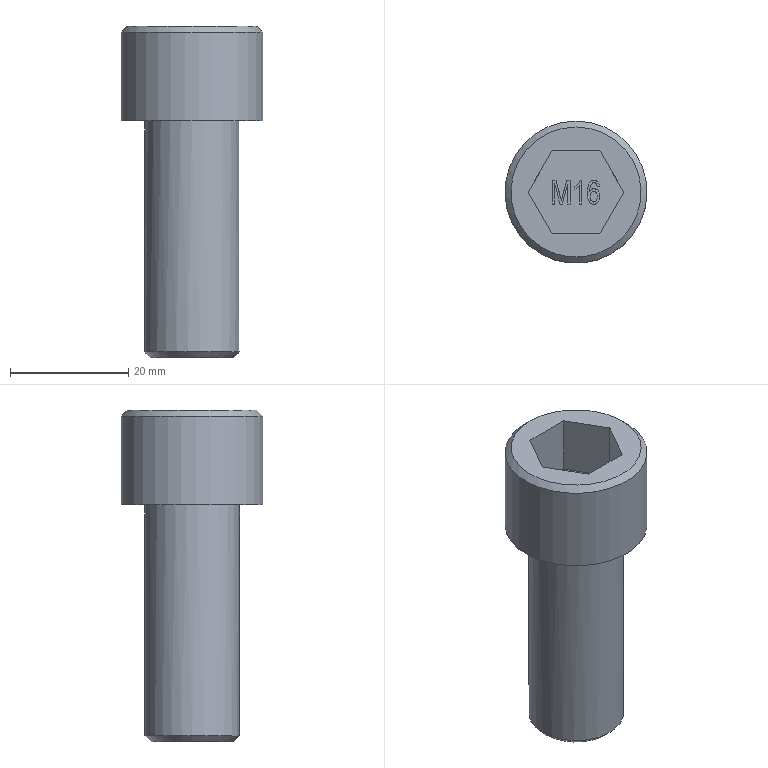Part | STEP file | M16-2 | 1 solid | 46 faces | box 24 x 24 x 56 mm | volume 13524 mm3 | plane 31 | other 11 | cylinder 2 | cone 2 | commonest cylinder face diameters 16 x1 24 x1